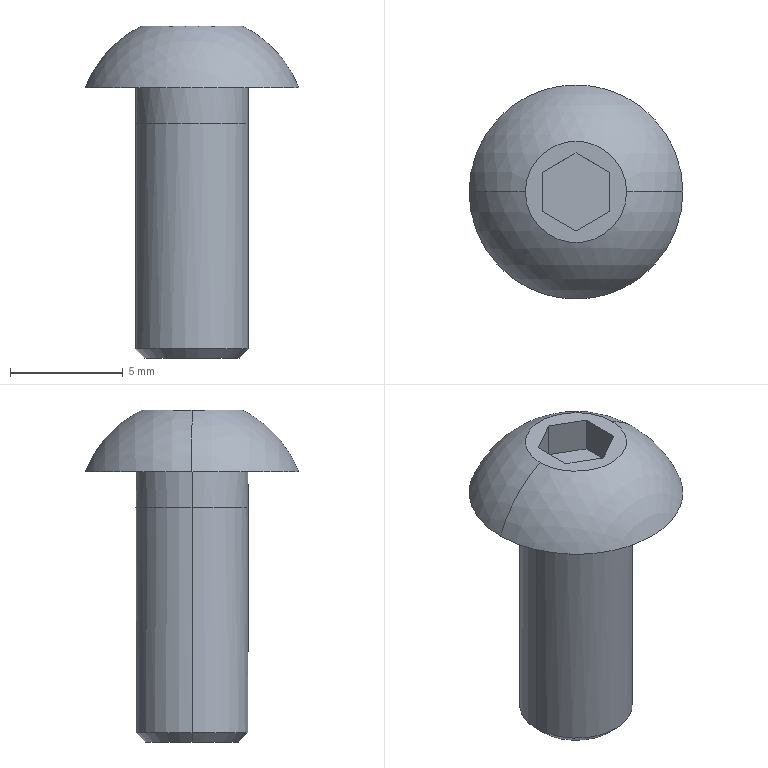Part | STEP file | button head socket screw ISO 7380 M5-12-A | 1 solid | 18 faces | box 9.5 x 9.5 x 14.75 mm | volume 352.491 mm3 | plane 10 | cylinder 4 | sphere 2 | cone 2 | commonest cylinder face diameters 5 x4
STEP:
#1=CARTESIAN_POINT('',(0.,0.,0.));
#2=DIRECTION('',(0.,0.,1.));
#3=DIRECTION('',(1.,0.,0.));
#4=AXIS2_PLACEMENT_3D('',#1,#2,#3);
#5=CARTESIAN_POINT('',(4.75,0.,0.));
#6=VERTEX_POINT('',#5);
#7=CARTESIAN_POINT('',(-4.75,0.,0.));
#8=VERTEX_POINT('',#7);
#9=CARTESIAN_POINT('',(0.,0.,0.));
#10=DIRECTION('',(0.,0.,1.));
#11=DIRECTION('',(1.,0.,0.));
#12=AXIS2_PLACEMENT_3D('',#9,#10,#11);
#13=CIRCLE('',#12,4.75);
#14=CARTESIAN_POINT('',(0.,0.,-1.807));
#15=DIRECTION('',(0.,1.,0.));
#16=DIRECTION('',(1.,0.,0.));
#17=AXIS2_PLACEMENT_3D('',#14,#15,#16);
#18=SPHERICAL_SURFACE('',#17,5.082);
#19=CARTESIAN_POINT('',(5.92,0.));
#20=CARTESIAN_POINT('',(5.92,0.04448));
#21=CARTESIAN_POINT('',(5.917,0.1335));
#22=CARTESIAN_POINT('',(5.907,0.2666));
#23=CARTESIAN_POINT('',(5.889,0.399));
#24=CARTESIAN_POINT('',(5.861,0.5301));
#25=CARTESIAN_POINT('',(5.82,0.6592));
#26=CARTESIAN_POINT('',(5.761,0.7852));
#27=CARTESIAN_POINT('',(5.677,0.9062));
#28=CARTESIAN_POINT('',(5.552,1.019));
#29=CARTESIAN_POINT('',(5.365,1.117));
#30=CARTESIAN_POINT('',(5.086,1.189));
#31=CARTESIAN_POINT('',(4.712,1.217));
#32=CARTESIAN_POINT('',(4.339,1.189));
#33=CARTESIAN_POINT('',(4.06,1.117));
#34=CARTESIAN_POINT('',(3.873,1.019));
#35=CARTESIAN_POINT('',(3.748,0.9062));
#36=CARTESIAN_POINT('',(3.663,0.7852));
#37=CARTESIAN_POINT('',(3.605,0.6592));
#38=CARTESIAN_POINT('',(3.564,0.5301));
#39=CARTESIAN_POINT('',(3.536,0.399));
#40=CARTESIAN_POINT('',(3.518,0.2666));
#41=CARTESIAN_POINT('',(3.507,0.1335));
#42=CARTESIAN_POINT('',(3.505,0.04448));
#43=CARTESIAN_POINT('',(3.505,0.));
#44=B_SPLINE_CURVE_WITH_KNOTS('',3,(#19,#20,#21,#22,#23,#24,#25,#26,#27,#28,#29,#30,#31,#32,#33,#34,#35,#36,#37,#38,#39,#40,#41,#42,#43),.UNSPECIFIED.,.F.,.F.,(4,1,1,1,1,1,1,1,1,1,1,1,1,1,1,1,1,1,1,1,1,1,4),(0.,0.1428,0.2856,0.4284,0.5712,0.714,0.8568,0.9996,1.142,1.285,1.428,1.571,1.714,1.856,1.999,2.142,2.285,2.428,2.57,2.713,2.856,2.999,3.142),.QUASI_UNIFORM_KNOTS.);
#45=(GEOMETRIC_REPRESENTATION_CONTEXT(2)PARAMETRIC_REPRESENTATION_CONTEXT()REPRESENTATION_CONTEXT('',''));
#46=DEFINITIONAL_REPRESENTATION('',(#44),#45);
#47=PCURVE('',#18,#46);
#48=CARTESIAN_POINT('',(2.5,0.,0.));
#49=DIRECTION('',(0.,0.,1.));
#50=DIRECTION('',(1.,0.,0.));
#51=AXIS2_PLACEMENT_3D('',#48,#49,#50);
#52=PLANE('',#51);
#53=CARTESIAN_POINT('',(-2.5,0.));
#54=DIRECTION('',(1.,0.));
#55=AXIS2_PLACEMENT_2D('',#53,#54);
#56=CIRCLE('',#55,4.75);
#57=(GEOMETRIC_REPRESENTATION_CONTEXT(2)PARAMETRIC_REPRESENTATION_CONTEXT()REPRESENTATION_CONTEXT('',''));
#58=DEFINITIONAL_REPRESENTATION('',(#56),#57);
#59=PCURVE('',#52,#58);
#60=SURFACE_CURVE('',#13,(#47,#59),.PCURVE_S1.);
#61=EDGE_CURVE('',#6,#8,#60,.T.);
#62=ORIENTED_EDGE('',*,*,#61,.T.);
#63=CARTESIAN_POINT('',(-2.25,0.,2.75));
#64=VERTEX_POINT('',#63);
#65=CARTESIAN_POINT('',(0.,0.,-1.807));
#66=DIRECTION('',(0.,1.,0.));
#67=DIRECTION('',(-1.,0.,0.));
#68=AXIS2_PLACEMENT_3D('',#65,#66,#67);
#69=CIRCLE('',#68,5.082);
#70=CARTESIAN_POINT('',(3.142,0.));
#71=DIRECTION('',(1.,0.));
#72=VECTOR('',#71,1.);
#73=LINE('',#70,#72);
#74=(GEOMETRIC_REPRESENTATION_CONTEXT(2)PARAMETRIC_REPRESENTATION_CONTEXT()REPRESENTATION_CONTEXT('',''));
#75=DEFINITIONAL_REPRESENTATION('',(#73),#74);
#76=PCURVE('',#18,#75);
#77=CARTESIAN_POINT('',(0.,0.,-1.807));
#78=DIRECTION('',(0.,1.,0.));
#79=DIRECTION('',(1.,0.,0.));
#80=AXIS2_PLACEMENT_3D('',#77,#78,#79);
#81=SPHERICAL_SURFACE('',#80,5.082);
#82=CARTESIAN_POINT('',(3.142,0.));
#83=DIRECTION('',(1.,0.));
#84=VECTOR('',#83,1.);
#85=LINE('',#82,#84);
#86=(GEOMETRIC_REPRESENTATION_CONTEXT(2)PARAMETRIC_REPRESENTATION_CONTEXT()REPRESENTATION_CONTEXT('',''));
#87=DEFINITIONAL_REPRESENTATION('',(#85),#86);
#88=PCURVE('',#81,#87);
#89=SURFACE_CURVE('',#69,(#76,#88),.PCURVE_S1.);
#90=EDGE_CURVE('',#8,#64,#89,.T.);
#91=ORIENTED_EDGE('',*,*,#90,.T.);
#92=CARTESIAN_POINT('',(2.25,0.,2.75));
#93=VERTEX_POINT('',#92);
#94=CARTESIAN_POINT('',(0.,0.,2.75));
#95=DIRECTION('',(0.,0.,1.));
#96=DIRECTION('',(1.,0.,0.));
#97=AXIS2_PLACEMENT_3D('',#94,#95,#96);
#98=CIRCLE('',#97,2.25);
#99=CARTESIAN_POINT('',(5.171,0.));
#100=CARTESIAN_POINT('',(5.171,0.02107));
#101=CARTESIAN_POINT('',(5.168,0.06322));
#102=CARTESIAN_POINT('',(5.156,0.1254));
#103=CARTESIAN_POINT('',(5.136,0.1855));
#104=CARTESIAN_POINT('',(5.107,0.2424));
#105=CARTESIAN_POINT('',(5.071,0.2951));
#106=CARTESIAN_POINT('',(5.026,0.3423));
#107=CARTESIAN_POINT('',(4.974,0.3829));
#108=CARTESIAN_POINT('',(4.916,0.4159));
#109=CARTESIAN_POINT('',(4.851,0.4403));
#110=CARTESIAN_POINT('',(4.783,0.4553));
#111=CARTESIAN_POINT('',(4.712,0.4603));
#112=CARTESIAN_POINT('',(4.642,0.4553));
#113=CARTESIAN_POINT('',(4.573,0.4403));
#114=CARTESIAN_POINT('',(4.509,0.4159));
#115=CARTESIAN_POINT('',(4.45,0.3829));
#116=CARTESIAN_POINT('',(4.398,0.3423));
#117=CARTESIAN_POINT('',(4.354,0.2951));
#118=CARTESIAN_POINT('',(4.317,0.2424));
#119=CARTESIAN_POINT('',(4.289,0.1855));
#120=CARTESIAN_POINT('',(4.269,0.1254));
#121=CARTESIAN_POINT('',(4.256,0.06322));
#122=CARTESIAN_POINT('',(4.254,0.02107));
#123=CARTESIAN_POINT('',(4.254,0.));
#124=B_SPLINE_CURVE_WITH_KNOTS('',3,(#99,#100,#101,#102,#103,#104,#105,#106,#107,#108,#109,#110,#111,#112,#113,#114,#115,#116,#117,#118,#119,#120,#121,#122,#123),.UNSPECIFIED.,.F.,.F.,(4,1,1,1,1,1,1,1,1,1,1,1,1,1,1,1,1,1,1,1,1,1,4),(0.,0.1428,0.2856,0.4284,0.5712,0.714,0.8568,0.9996,1.142,1.285,1.428,1.571,1.714,1.856,1.999,2.142,2.285,2.428,2.57,2.713,2.856,2.999,3.142),.QUASI_UNIFORM_KNOTS.);
#125=(GEOMETRIC_REPRESENTATION_CONTEXT(2)PARAMETRIC_REPRESENTATION_CONTEXT()REPRESENTATION_CONTEXT('',''));
#126=DEFINITIONAL_REPRESENTATION('',(#124),#125);
#127=PCURVE('',#18,#126);
#128=CARTESIAN_POINT('',(2.25,0.,2.75));
#129=DIRECTION('',(0.,0.,-1.));
#130=DIRECTION('',(-1.,0.,0.));
#131=AXIS2_PLACEMENT_3D('',#128,#129,#130);
#132=PLANE('',#131);
#133=CARTESIAN_POINT('',(0.,0.));
#134=CARTESIAN_POINT('',(0.,3.897));
#135=CARTESIAN_POINT('',(3.375,1.949));
#136=CARTESIAN_POINT('',(6.75,0.));
#137=CARTESIAN_POINT('',(3.375,-1.949));
#138=CARTESIAN_POINT('',(0.,-3.897));
#139=CARTESIAN_POINT('',(0.,0.));
#140=(BOUNDED_CURVE()B_SPLINE_CURVE(2,(#133,#134,#135,#136,#137,#138,#139),.UNSPECIFIED.,.T.,.F.)B_SPLINE_CURVE_WITH_KNOTS((1,2,2,2,2,1),(-2.094,0.,2.094,4.189,6.283,8.378),.UNSPECIFIED.)CURVE()GEOMETRIC_REPRESENTATION_ITEM()RATIONAL_B_SPLINE_CURVE((1.,0.5,1.,0.5,1.,0.5,1.))REPRESENTATION_ITEM(''));
#141=(GEOMETRIC_REPRESENTATION_CONTEXT(2)PARAMETRIC_REPRESENTATION_CONTEXT()REPRESENTATION_CONTEXT('',''));
#142=DEFINITIONAL_REPRESENTATION('',(#140),#141);
#143=PCURVE('',#132,#142);
#144=SURFACE_CURVE('',#98,(#127,#143),.PCURVE_S1.);
#145=EDGE_CURVE('',#93,#64,#144,.T.);
#146=ORIENTED_EDGE('',*,*,#145,.F.);
#147=CARTESIAN_POINT('',(0.,0.,-1.807));
#148=DIRECTION('',(0.,-1.,0.));
#149=DIRECTION('',(0.,0.,-1.));
#150=AXIS2_PLACEMENT_3D('',#147,#148,#149);
#151=CIRCLE('',#150,5.082);
#152=CARTESIAN_POINT('',(7.854,0.));
#153=DIRECTION('',(-1.,0.));
#154=VECTOR('',#153,1.);
#155=LINE('',#152,#154);
#156=(GEOMETRIC_REPRESENTATION_CONTEXT(2)PARAMETRIC_REPRESENTATION_CONTEXT()REPRESENTATION_CONTEXT('',''));
#157=DEFINITIONAL_REPRESENTATION('',(#155),#156);
#158=PCURVE('',#18,#157);
#159=CARTESIAN_POINT('',(7.854,0.));
#160=DIRECTION('',(-1.,0.));
#161=VECTOR('',#160,1.);
#162=LINE('',#159,#161);
#163=(GEOMETRIC_REPRESENTATION_CONTEXT(2)PARAMETRIC_REPRESENTATION_CONTEXT()REPRESENTATION_CONTEXT('',''));
#164=DEFINITIONAL_REPRESENTATION('',(#162),#163);
#165=PCURVE('',#81,#164);
#166=SURFACE_CURVE('',#151,(#158,#165),.PCURVE_S1.);
#167=EDGE_CURVE('',#6,#93,#166,.T.);
#168=ORIENTED_EDGE('',*,*,#167,.F.);
#169=EDGE_LOOP('',(#62,#91,#146,#168));
#170=FACE_BOUND('',#169,.T.);
#171=ADVANCED_FACE('',(#170),#18,.T.);
#172=CARTESIAN_POINT('',(-2.5,0.,-1.6));
#173=VERTEX_POINT('',#172);
#174=CARTESIAN_POINT('',(2.5,0.,-1.6));
#175=VERTEX_POINT('',#174);
#176=CARTESIAN_POINT('',(-2.5,0.,-1.6));
#177=CARTESIAN_POINT('',(-2.5,0.3272,-1.6));
#178=CARTESIAN_POINT('',(-2.435,0.6544,-1.6));
#179=CARTESIAN_POINT('',(-2.184,1.259,-1.6));
#180=CARTESIAN_POINT('',(-1.999,1.536,-1.6));
#181=CARTESIAN_POINT('',(-1.536,1.999,-1.6));
#182=CARTESIAN_POINT('',(-1.259,2.184,-1.6));
#183=CARTESIAN_POINT('',(-0.6544,2.435,-1.6));
#184=CARTESIAN_POINT('',(-0.3272,2.5,-1.6));
#185=CARTESIAN_POINT('',(0.3272,2.5,-1.6));
#186=CARTESIAN_POINT('',(0.6544,2.435,-1.6));
#187=CARTESIAN_POINT('',(1.259,2.184,-1.6));
#188=CARTESIAN_POINT('',(1.536,1.999,-1.6));
#189=CARTESIAN_POINT('',(1.999,1.536,-1.6));
#190=CARTESIAN_POINT('',(2.184,1.259,-1.6));
#191=CARTESIAN_POINT('',(2.435,0.6544,-1.6));
#192=CARTESIAN_POINT('',(2.5,0.3272,-1.6));
#193=CARTESIAN_POINT('',(2.5,0.,-1.6));
#194=B_SPLINE_CURVE_WITH_KNOTS('',3,(#176,#177,#178,#179,#180,#181,#182,#183,#184,#185,#186,#187,#188,#189,#190,#191,#192,#193),.UNSPECIFIED.,.F.,.F.,(4,2,2,2,2,2,2,2,4),(0.5,0.5625,0.625,0.6875,0.75,0.8125,0.875,0.9375,1.),.UNSPECIFIED.);
#195=CARTESIAN_POINT('',(0.,0.,2.75));
#196=DIRECTION('',(0.,0.,1.));
#197=DIRECTION('',(1.,0.,0.));
#198=AXIS2_PLACEMENT_3D('',#195,#196,#197);
#199=CYLINDRICAL_SURFACE('',#198,2.5);
#200=CARTESIAN_POINT('',(3.142,-4.35));
#201=CARTESIAN_POINT('',(0.,-4.35));
#202=B_SPLINE_CURVE_WITH_KNOTS('',1,(#200,#201),.UNSPECIFIED.,.F.,.F.,(2,2),(0.5,1.),.PIECEWISE_BEZIER_KNOTS.);
#203=(GEOMETRIC_REPRESENTATION_CONTEXT(2)PARAMETRIC_REPRESENTATION_CONTEXT()REPRESENTATION_CONTEXT('',''));
#204=DEFINITIONAL_REPRESENTATION('',(#202),#203);
#205=PCURVE('',#199,#204);
#206=CARTESIAN_POINT('',(0.,0.,2.75));
#207=DIRECTION('',(0.,0.,1.));
#208=DIRECTION('',(1.,0.,0.));
#209=AXIS2_PLACEMENT_3D('',#206,#207,#208);
#210=CYLINDRICAL_SURFACE('',#209,2.5);
#211=CARTESIAN_POINT('',(3.142,-4.35));
#212=CARTESIAN_POINT('',(0.,-4.35));
#213=B_SPLINE_CURVE_WITH_KNOTS('',1,(#211,#212),.UNSPECIFIED.,.F.,.F.,(2,2),(0.5,1.),.PIECEWISE_BEZIER_KNOTS.);
#214=(GEOMETRIC_REPRESENTATION_CONTEXT(2)PARAMETRIC_REPRESENTATION_CONTEXT()REPRESENTATION_CONTEXT('',''));
#215=DEFINITIONAL_REPRESENTATION('',(#213),#214);
#216=PCURVE('',#210,#215);
#217=SURFACE_CURVE('',#194,(#205,#216),.PCURVE_S1.);
#218=EDGE_CURVE('',#173,#175,#217,.T.);
#219=ORIENTED_EDGE('',*,*,#218,.F.);
#220=CARTESIAN_POINT('',(-2.5,0.,0.));
#221=VERTEX_POINT('',#220);
#222=CARTESIAN_POINT('',(-2.5,0.,2.75));
#223=DIRECTION('',(0.,0.,1.));
#224=VECTOR('',#223,1.);
#225=LINE('',#222,#224);
#226=CARTESIAN_POINT('',(3.142,0.));
#227=DIRECTION('',(0.,1.));
#228=VECTOR('',#227,1.);
#229=LINE('',#226,#228);
#230=(GEOMETRIC_REPRESENTATION_CONTEXT(2)PARAMETRIC_REPRESENTATION_CONTEXT()REPRESENTATION_CONTEXT('',''));
#231=DEFINITIONAL_REPRESENTATION('',(#229),#230);
#232=PCURVE('',#199,#231);
#233=CARTESIAN_POINT('',(0.,0.,2.75));
#234=DIRECTION('',(0.,0.,1.));
#235=DIRECTION('',(1.,0.,0.));
#236=AXIS2_PLACEMENT_3D('',#233,#234,#235);
#237=CYLINDRICAL_SURFACE('',#236,2.5);
#238=CARTESIAN_POINT('',(3.142,0.));
#239=DIRECTION('',(0.,1.));
#240=VECTOR('',#239,1.);
#241=LINE('',#238,#240);
#242=(GEOMETRIC_REPRESENTATION_CONTEXT(2)PARAMETRIC_REPRESENTATION_CONTEXT()REPRESENTATION_CONTEXT('',''));
#243=DEFINITIONAL_REPRESENTATION('',(#241),#242);
#244=PCURVE('',#237,#243);
#245=SURFACE_CURVE('',#225,(#232,#244),.PCURVE_S1.);
#246=EDGE_CURVE('',#173,#221,#245,.T.);
#247=ORIENTED_EDGE('',*,*,#246,.T.);
#248=CARTESIAN_POINT('',(2.5,0.,0.));
#249=VERTEX_POINT('',#248);
#250=CARTESIAN_POINT('',(0.,0.,0.));
#251=DIRECTION('',(0.,0.,1.));
#252=DIRECTION('',(1.,0.,0.));
#253=AXIS2_PLACEMENT_3D('',#250,#251,#252);
#254=CIRCLE('',#253,2.5);
#255=CARTESIAN_POINT('',(0.,-2.75));
#256=DIRECTION('',(1.,0.));
#257=VECTOR('',#256,1.);
#258=LINE('',#255,#257);
#259=(GEOMETRIC_REPRESENTATION_CONTEXT(2)PARAMETRIC_REPRESENTATION_CONTEXT()REPRESENTATION_CONTEXT('',''));
#260=DEFINITIONAL_REPRESENTATION('',(#258),#259);
#261=PCURVE('',#199,#260);
#262=CARTESIAN_POINT('',(-2.5,0.));
#263=DIRECTION('',(1.,0.));
#264=AXIS2_PLACEMENT_2D('',#262,#263);
#265=CIRCLE('',#264,2.5);
#266=(GEOMETRIC_REPRESENTATION_CONTEXT(2)PARAMETRIC_REPRESENTATION_CONTEXT()REPRESENTATION_CONTEXT('',''));
#267=DEFINITIONAL_REPRESENTATION('',(#265),#266);
#268=PCURVE('',#52,#267);
#269=SURFACE_CURVE('',#254,(#261,#268),.PCURVE_S1.);
#270=EDGE_CURVE('',#249,#221,#269,.T.);
#271=ORIENTED_EDGE('',*,*,#270,.F.);
#272=CARTESIAN_POINT('',(2.5,0.,2.75));
#273=DIRECTION('',(0.,0.,1.));
#274=VECTOR('',#273,1.);
#275=LINE('',#272,#274);
#276=CARTESIAN_POINT('',(0.,0.));
#277=DIRECTION('',(0.,1.));
#278=VECTOR('',#277,1.);
#279=LINE('',#276,#278);
#280=(GEOMETRIC_REPRESENTATION_CONTEXT(2)PARAMETRIC_REPRESENTATION_CONTEXT()REPRESENTATION_CONTEXT('',''));
#281=DEFINITIONAL_REPRESENTATION('',(#279),#280);
#282=PCURVE('',#199,#281);
#283=CARTESIAN_POINT('',(6.283,0.));
#284=DIRECTION('',(0.,1.));
#285=VECTOR('',#284,1.);
#286=LINE('',#283,#285);
#287=(GEOMETRIC_REPRESENTATION_CONTEXT(2)PARAMETRIC_REPRESENTATION_CONTEXT()REPRESENTATION_CONTEXT('',''));
#288=DEFINITIONAL_REPRESENTATION('',(#286),#287);
#289=PCURVE('',#237,#288);
#290=SURFACE_CURVE('',#275,(#282,#289),.PCURVE_S1.);
#291=EDGE_CURVE('',#175,#249,#290,.T.);
#292=ORIENTED_EDGE('',*,*,#291,.F.);
#293=EDGE_LOOP('',(#219,#247,#271,#292));
#294=FACE_BOUND('',#293,.T.);
#295=ADVANCED_FACE('',(#294),#199,.T.);
#296=CARTESIAN_POINT('',(2.1,0.,-12.));
#297=VERTEX_POINT('',#296);
#298=CARTESIAN_POINT('',(-2.1,0.,-12.));
#299=VERTEX_POINT('',#298);
#300=CARTESIAN_POINT('',(0.,0.,-12.));
#301=DIRECTION('',(0.,0.,1.));
#302=DIRECTION('',(1.,0.,0.));
#303=AXIS2_PLACEMENT_3D('',#300,#301,#302);
#304=CIRCLE('',#303,2.1);
#305=CARTESIAN_POINT('',(0.,0.,-12.));
#306=DIRECTION('',(0.,0.,1.));
#307=DIRECTION('',(1.,0.,0.));
#308=AXIS2_PLACEMENT_3D('',#305,#306,#307);
#309=CONICAL_SURFACE('',#308,2.1,0.7854);
#310=CARTESIAN_POINT('',(0.,0.));
#311=DIRECTION('',(1.,0.));
#312=VECTOR('',#311,1.);
#313=LINE('',#310,#312);
#314=(GEOMETRIC_REPRESENTATION_CONTEXT(2)PARAMETRIC_REPRESENTATION_CONTEXT()REPRESENTATION_CONTEXT('',''));
#315=DEFINITIONAL_REPRESENTATION('',(#313),#314);
#316=PCURVE('',#309,#315);
#317=CARTESIAN_POINT('',(0.,0.,-12.));
#318=DIRECTION('',(0.,0.,1.));
#319=DIRECTION('',(1.,0.,0.));
#320=AXIS2_PLACEMENT_3D('',#317,#318,#319);
#321=PLANE('',#320);
#322=CARTESIAN_POINT('',(0.,0.));
#323=DIRECTION('',(1.,0.));
#324=AXIS2_PLACEMENT_2D('',#322,#323);
#325=CIRCLE('',#324,2.1);
#326=(GEOMETRIC_REPRESENTATION_CONTEXT(2)PARAMETRIC_REPRESENTATION_CONTEXT()REPRESENTATION_CONTEXT('',''));
#327=DEFINITIONAL_REPRESENTATION('',(#325),#326);
#328=PCURVE('',#321,#327);
#329=SURFACE_CURVE('',#304,(#316,#328),.PCURVE_S1.);
#330=EDGE_CURVE('',#297,#299,#329,.T.);
#331=ORIENTED_EDGE('',*,*,#330,.T.);
#332=CARTESIAN_POINT('',(-2.5,0.,-11.6));
#333=VERTEX_POINT('',#332);
#334=CARTESIAN_POINT('',(-2.1,0.,-12.));
#335=DIRECTION('',(-0.7071,0.,0.7071));
#336=VECTOR('',#335,1.);
#337=LINE('',#334,#336);
#338=CARTESIAN_POINT('',(3.142,0.));
#339=DIRECTION('',(0.,1.));
#340=VECTOR('',#339,1.);
#341=LINE('',#338,#340);
#342=(GEOMETRIC_REPRESENTATION_CONTEXT(2)PARAMETRIC_REPRESENTATION_CONTEXT()REPRESENTATION_CONTEXT('',''));
#343=DEFINITIONAL_REPRESENTATION('',(#341),#342);
#344=PCURVE('',#309,#343);
#345=CARTESIAN_POINT('',(0.,0.,-12.));
#346=DIRECTION('',(0.,0.,1.));
#347=DIRECTION('',(1.,0.,0.));
#348=AXIS2_PLACEMENT_3D('',#345,#346,#347);
#349=CONICAL_SURFACE('',#348,2.1,0.7854);
#350=CARTESIAN_POINT('',(3.142,0.));
#351=DIRECTION('',(0.,1.));
#352=VECTOR('',#351,1.);
#353=LINE('',#350,#352);
#354=(GEOMETRIC_REPRESENTATION_CONTEXT(2)PARAMETRIC_REPRESENTATION_CONTEXT()REPRESENTATION_CONTEXT('',''));
#355=DEFINITIONAL_REPRESENTATION('',(#353),#354);
#356=PCURVE('',#349,#355);
#357=SURFACE_CURVE('',#337,(#344,#356),.PCURVE_S1.);
#358=EDGE_CURVE('',#299,#333,#357,.T.);
#359=ORIENTED_EDGE('',*,*,#358,.T.);
#360=CARTESIAN_POINT('',(2.5,0.,-11.6));
#361=VERTEX_POINT('',#360);
#362=CARTESIAN_POINT('',(0.,0.,-11.6));
#363=DIRECTION('',(0.,0.,1.));
#364=DIRECTION('',(1.,0.,0.));
#365=AXIS2_PLACEMENT_3D('',#362,#363,#364);
#366=CIRCLE('',#365,2.5);
#367=CARTESIAN_POINT('',(0.,0.4));
#368=DIRECTION('',(1.,0.));
#369=VECTOR('',#368,1.);
#370=LINE('',#367,#369);
#371=(GEOMETRIC_REPRESENTATION_CONTEXT(2)PARAMETRIC_REPRESENTATION_CONTEXT()REPRESENTATION_CONTEXT('',''));
#372=DEFINITIONAL_REPRESENTATION('',(#370),#371);
#373=PCURVE('',#309,#372);
#374=CARTESIAN_POINT('',(0.,-14.35));
#375=DIRECTION('',(1.,0.));
#376=VECTOR('',#375,1.);
#377=LINE('',#374,#376);
#378=(GEOMETRIC_REPRESENTATION_CONTEXT(2)PARAMETRIC_REPRESENTATION_CONTEXT()REPRESENTATION_CONTEXT('',''));
#379=DEFINITIONAL_REPRESENTATION('',(#377),#378);
#380=PCURVE('',#210,#379);
#381=SURFACE_CURVE('',#366,(#373,#380),.PCURVE_S1.);
#382=EDGE_CURVE('',#361,#333,#381,.T.);
#383=ORIENTED_EDGE('',*,*,#382,.F.);
#384=CARTESIAN_POINT('',(2.1,0.,-12.));
#385=DIRECTION('',(0.7071,0.,0.7071));
#386=VECTOR('',#385,1.);
#387=LINE('',#384,#386);
#388=CARTESIAN_POINT('',(0.,0.));
#389=DIRECTION('',(0.,1.));
#390=VECTOR('',#389,1.);
#391=LINE('',#388,#390);
#392=(GEOMETRIC_REPRESENTATION_CONTEXT(2)PARAMETRIC_REPRESENTATION_CONTEXT()REPRESENTATION_CONTEXT('',''));
#393=DEFINITIONAL_REPRESENTATION('',(#391),#392);
#394=PCURVE('',#309,#393);
#395=CARTESIAN_POINT('',(6.283,0.));
#396=DIRECTION('',(0.,1.));
#397=VECTOR('',#396,1.);
#398=LINE('',#395,#397);
#399=(GEOMETRIC_REPRESENTATION_CONTEXT(2)PARAMETRIC_REPRESENTATION_CONTEXT()REPRESENTATION_CONTEXT('',''));
#400=DEFINITIONAL_REPRESENTATION('',(#398),#399);
#401=PCURVE('',#349,#400);
#402=SURFACE_CURVE('',#387,(#394,#401),.PCURVE_S1.);
#403=EDGE_CURVE('',#297,#361,#402,.T.);
#404=ORIENTED_EDGE('',*,*,#403,.F.);
#405=EDGE_LOOP('',(#331,#359,#383,#404));
#406=FACE_BOUND('',#405,.T.);
#407=ADVANCED_FACE('',(#406),#309,.T.);
#408=ORIENTED_EDGE('',*,*,#382,.T.);
#409=CARTESIAN_POINT('',(-2.5,0.,2.75));
#410=DIRECTION('',(0.,0.,1.));
#411=VECTOR('',#410,1.);
#412=LINE('',#409,#411);
#413=CARTESIAN_POINT('',(3.142,0.));
#414=DIRECTION('',(0.,1.));
#415=VECTOR('',#414,1.);
#416=LINE('',#413,#415);
#417=(GEOMETRIC_REPRESENTATION_CONTEXT(2)PARAMETRIC_REPRESENTATION_CONTEXT()REPRESENTATION_CONTEXT('',''));
#418=DEFINITIONAL_REPRESENTATION('',(#416),#417);
#419=PCURVE('',#210,#418);
#420=CARTESIAN_POINT('',(0.,0.,2.75));
#421=DIRECTION('',(0.,0.,1.));
#422=DIRECTION('',(1.,0.,0.));
#423=AXIS2_PLACEMENT_3D('',#420,#421,#422);
#424=CYLINDRICAL_SURFACE('',#423,2.5);
#425=CARTESIAN_POINT('',(3.142,0.));
#426=DIRECTION('',(0.,1.));
#427=VECTOR('',#426,1.);
#428=LINE('',#425,#427);
#429=(GEOMETRIC_REPRESENTATION_CONTEXT(2)PARAMETRIC_REPRESENTATION_CONTEXT()REPRESENTATION_CONTEXT('',''));
#430=DEFINITIONAL_REPRESENTATION('',(#428),#429);
#431=PCURVE('',#424,#430);
#432=SURFACE_CURVE('',#412,(#419,#431),.PCURVE_S1.);
#433=EDGE_CURVE('',#333,#173,#432,.T.);
#434=ORIENTED_EDGE('',*,*,#433,.T.);
#435=ORIENTED_EDGE('',*,*,#218,.T.);
#436=CARTESIAN_POINT('',(2.5,0.,2.75));
#437=DIRECTION('',(0.,0.,1.));
#438=VECTOR('',#437,1.);
#439=LINE('',#436,#438);
#440=CARTESIAN_POINT('',(0.,0.));
#441=DIRECTION('',(0.,1.));
#442=VECTOR('',#441,1.);
#443=LINE('',#440,#442);
#444=(GEOMETRIC_REPRESENTATION_CONTEXT(2)PARAMETRIC_REPRESENTATION_CONTEXT()REPRESENTATION_CONTEXT('',''));
#445=DEFINITIONAL_REPRESENTATION('',(#443),#444);
#446=PCURVE('',#210,#445);
#447=CARTESIAN_POINT('',(6.283,0.));
#448=DIRECTION('',(0.,1.));
#449=VECTOR('',#448,1.);
#450=LINE('',#447,#449);
#451=(GEOMETRIC_REPRESENTATION_CONTEXT(2)PARAMETRIC_REPRESENTATION_CONTEXT()REPRESENTATION_CONTEXT('',''));
#452=DEFINITIONAL_REPRESENTATION('',(#450),#451);
#453=PCURVE('',#424,#452);
#454=SURFACE_CURVE('',#439,(#446,#453),.PCURVE_S1.);
#455=EDGE_CURVE('',#361,#175,#454,.T.);
#456=ORIENTED_EDGE('',*,*,#455,.F.);
#457=EDGE_LOOP('',(#408,#434,#435,#456));
#458=FACE_BOUND('',#457,.T.);
#459=ADVANCED_FACE('',(#458),#210,.T.);
#460=ORIENTED_EDGE('',*,*,#433,.F.);
#461=CARTESIAN_POINT('',(0.,0.,-11.6));
#462=DIRECTION('',(0.,0.,1.));
#463=DIRECTION('',(1.,0.,0.));
#464=AXIS2_PLACEMENT_3D('',#461,#462,#463);
#465=CIRCLE('',#464,2.5);
#466=CARTESIAN_POINT('',(0.,-14.35));
#467=DIRECTION('',(1.,0.));
#468=VECTOR('',#467,1.);
#469=LINE('',#466,#468);
#470=(GEOMETRIC_REPRESENTATION_CONTEXT(2)PARAMETRIC_REPRESENTATION_CONTEXT()REPRESENTATION_CONTEXT('',''));
#471=DEFINITIONAL_REPRESENTATION('',(#469),#470);
#472=PCURVE('',#424,#471);
#473=CARTESIAN_POINT('',(0.,0.4));
#474=DIRECTION('',(1.,0.));
#475=VECTOR('',#474,1.);
#476=LINE('',#473,#475);
#477=(GEOMETRIC_REPRESENTATION_CONTEXT(2)PARAMETRIC_REPRESENTATION_CONTEXT()REPRESENTATION_CONTEXT('',''));
#478=DEFINITIONAL_REPRESENTATION('',(#476),#477);
#479=PCURVE('',#349,#478);
#480=SURFACE_CURVE('',#465,(#472,#479),.PCURVE_S1.);
#481=EDGE_CURVE('',#333,#361,#480,.T.);
#482=ORIENTED_EDGE('',*,*,#481,.T.);
#483=ORIENTED_EDGE('',*,*,#455,.T.);
#484=CARTESIAN_POINT('',(2.5,0.,-1.6));
#485=CARTESIAN_POINT('',(2.5,-0.3272,-1.6));
#486=CARTESIAN_POINT('',(2.435,-0.6544,-1.6));
#487=CARTESIAN_POINT('',(2.184,-1.259,-1.6));
#488=CARTESIAN_POINT('',(1.999,-1.536,-1.6));
#489=CARTESIAN_POINT('',(1.536,-1.999,-1.6));
#490=CARTESIAN_POINT('',(1.259,-2.184,-1.6));
#491=CARTESIAN_POINT('',(0.6544,-2.435,-1.6));
#492=CARTESIAN_POINT('',(0.3272,-2.5,-1.6));
#493=CARTESIAN_POINT('',(-0.3272,-2.5,-1.6));
#494=CARTESIAN_POINT('',(-0.6544,-2.435,-1.6));
#495=CARTESIAN_POINT('',(-1.259,-2.184,-1.6));
#496=CARTESIAN_POINT('',(-1.536,-1.999,-1.6));
#497=CARTESIAN_POINT('',(-1.999,-1.536,-1.6));
#498=CARTESIAN_POINT('',(-2.184,-1.259,-1.6));
#499=CARTESIAN_POINT('',(-2.435,-0.6544,-1.6));
#500=CARTESIAN_POINT('',(-2.5,-0.3272,-1.6));
#501=CARTESIAN_POINT('',(-2.5,0.,-1.6));
#502=B_SPLINE_CURVE_WITH_KNOTS('',3,(#484,#485,#486,#487,#488,#489,#490,#491,#492,#493,#494,#495,#496,#497,#498,#499,#500,#501),.UNSPECIFIED.,.F.,.F.,(4,2,2,2,2,2,2,2,4),(0.,0.0625,0.125,0.1875,0.25,0.3125,0.375,0.4375,0.5),.UNSPECIFIED.);
#503=CARTESIAN_POINT('',(6.283,-4.35));
#504=CARTESIAN_POINT('',(3.142,-4.35));
#505=B_SPLINE_CURVE_WITH_KNOTS('',1,(#503,#504),.UNSPECIFIED.,.F.,.F.,(2,2),(0.,0.5),.PIECEWISE_BEZIER_KNOTS.);
#506=(GEOMETRIC_REPRESENTATION_CONTEXT(2)PARAMETRIC_REPRESENTATION_CONTEXT()REPRESENTATION_CONTEXT('',''));
#507=DEFINITIONAL_REPRESENTATION('',(#505),#506);
#508=PCURVE('',#424,#507);
#509=CARTESIAN_POINT('',(6.283,-4.35));
#510=CARTESIAN_POINT('',(3.142,-4.35));
#511=B_SPLINE_CURVE_WITH_KNOTS('',1,(#509,#510),.UNSPECIFIED.,.F.,.F.,(2,2),(0.,0.5),.PIECEWISE_BEZIER_KNOTS.);
#512=(GEOMETRIC_REPRESENTATION_CONTEXT(2)PARAMETRIC_REPRESENTATION_CONTEXT()REPRESENTATION_CONTEXT('',''));
#513=DEFINITIONAL_REPRESENTATION('',(#511),#512);
#514=PCURVE('',#237,#513);
#515=SURFACE_CURVE('',#502,(#508,#514),.PCURVE_S1.);
#516=EDGE_CURVE('',#175,#173,#515,.T.);
#517=ORIENTED_EDGE('',*,*,#516,.T.);
#518=EDGE_LOOP('',(#460,#482,#483,#517));
#519=FACE_BOUND('',#518,.T.);
#520=ADVANCED_FACE('',(#519),#424,.T.);
#521=ORIENTED_EDGE('',*,*,#145,.T.);
#522=CARTESIAN_POINT('',(0.,0.,2.75));
#523=DIRECTION('',(0.,0.,1.));
#524=DIRECTION('',(1.,0.,0.));
#525=AXIS2_PLACEMENT_3D('',#522,#523,#524);
#526=CIRCLE('',#525,2.25);
#527=CARTESIAN_POINT('',(0.,0.));
#528=CARTESIAN_POINT('',(0.,3.897));
#529=CARTESIAN_POINT('',(3.375,1.949));
#530=CARTESIAN_POINT('',(6.75,0.));
#531=CARTESIAN_POINT('',(3.375,-1.949));
#532=CARTESIAN_POINT('',(0.,-3.897));
#533=CARTESIAN_POINT('',(0.,0.));
#534=(BOUNDED_CURVE()B_SPLINE_CURVE(2,(#527,#528,#529,#530,#531,#532,#533),.UNSPECIFIED.,.T.,.F.)B_SPLINE_CURVE_WITH_KNOTS((1,2,2,2,2,1),(-2.094,0.,2.094,4.189,6.283,8.378),.UNSPECIFIED.)CURVE()GEOMETRIC_REPRESENTATION_ITEM()RATIONAL_B_SPLINE_CURVE((1.,0.5,1.,0.5,1.,0.5,1.))REPRESENTATION_ITEM(''));
#535=(GEOMETRIC_REPRESENTATION_CONTEXT(2)PARAMETRIC_REPRESENTATION_CONTEXT()REPRESENTATION_CONTEXT('',''));
#536=DEFINITIONAL_REPRESENTATION('',(#534),#535);
#537=PCURVE('',#132,#536);
#538=CARTESIAN_POINT('',(4.254,0.));
#539=CARTESIAN_POINT('',(4.254,-0.02107));
#540=CARTESIAN_POINT('',(4.256,-0.06322));
#541=CARTESIAN_POINT('',(4.269,-0.1254));
#542=CARTESIAN_POINT('',(4.289,-0.1855));
#543=CARTESIAN_POINT('',(4.317,-0.2424));
#544=CARTESIAN_POINT('',(4.354,-0.2951));
#545=CARTESIAN_POINT('',(4.398,-0.3423));
#546=CARTESIAN_POINT('',(4.45,-0.3829));
#547=CARTESIAN_POINT('',(4.509,-0.4159));
#548=CARTESIAN_POINT('',(4.573,-0.4403));
#549=CARTESIAN_POINT('',(4.642,-0.4553));
#550=CARTESIAN_POINT('',(4.712,-0.4603));
#551=CARTESIAN_POINT('',(4.783,-0.4553));
#552=CARTESIAN_POINT('',(4.851,-0.4403));
#553=CARTESIAN_POINT('',(4.916,-0.4159));
#554=CARTESIAN_POINT('',(4.974,-0.3829));
#555=CARTESIAN_POINT('',(5.026,-0.3423));
#556=CARTESIAN_POINT('',(5.071,-0.2951));
#557=CARTESIAN_POINT('',(5.107,-0.2424));
#558=CARTESIAN_POINT('',(5.136,-0.1855));
#559=CARTESIAN_POINT('',(5.156,-0.1254));
#560=CARTESIAN_POINT('',(5.168,-0.06322));
#561=CARTESIAN_POINT('',(5.171,-0.02107));
#562=CARTESIAN_POINT('',(5.171,0.));
#563=B_SPLINE_CURVE_WITH_KNOTS('',3,(#538,#539,#540,#541,#542,#543,#544,#545,#546,#547,#548,#549,#550,#551,#552,#553,#554,#555,#556,#557,#558,#559,#560,#561,#562),.UNSPECIFIED.,.F.,.F.,(4,1,1,1,1,1,1,1,1,1,1,1,1,1,1,1,1,1,1,1,1,1,4),(3.142,3.284,3.427,3.57,3.713,3.856,3.998,4.141,4.284,4.427,4.57,4.712,4.855,4.998,5.141,5.284,5.426,5.569,5.712,5.855,5.998,6.14,6.283),.QUASI_UNIFORM_KNOTS.);
#564=(GEOMETRIC_REPRESENTATION_CONTEXT(2)PARAMETRIC_REPRESENTATION_CONTEXT()REPRESENTATION_CONTEXT('',''));
#565=DEFINITIONAL_REPRESENTATION('',(#563),#564);
#566=PCURVE('',#81,#565);
#567=SURFACE_CURVE('',#526,(#537,#566),.PCURVE_S1.);
#568=EDGE_CURVE('',#64,#93,#567,.T.);
#569=ORIENTED_EDGE('',*,*,#568,.T.);
#570=EDGE_LOOP('',(#521,#569));
#571=FACE_BOUND('',#570,.T.);
#572=CARTESIAN_POINT('',(1.5,-0.866,2.75));
#573=VERTEX_POINT('',#572);
#574=CARTESIAN_POINT('',(1.5,0.866,2.75));
#575=VERTEX_POINT('',#574);
#576=CARTESIAN_POINT('',(1.5,0.,2.75));
#577=DIRECTION('',(0.,1.,0.));
#578=VECTOR('',#577,1.);
#579=LINE('',#576,#578);
#580=CARTESIAN_POINT('',(0.75,0.));
#581=DIRECTION('',(0.,1.));
#582=VECTOR('',#581,1.);
#583=LINE('',#580,#582);
#584=(GEOMETRIC_REPRESENTATION_CONTEXT(2)PARAMETRIC_REPRESENTATION_CONTEXT()REPRESENTATION_CONTEXT('',''));
#585=DEFINITIONAL_REPRESENTATION('',(#583),#584);
#586=PCURVE('',#132,#585);
#587=CARTESIAN_POINT('',(1.5,-0.866,21.142));
#588=DIRECTION('',(-1.,0.,0.));
#589=DIRECTION('',(0.,-1.,0.));
#590=AXIS2_PLACEMENT_3D('',#587,#588,#589);
#591=PLANE('',#590);
#592=CARTESIAN_POINT('',(-0.866,-18.392));
#593=DIRECTION('',(-1.,0.));
#594=VECTOR('',#593,1.);
#595=LINE('',#592,#594);
#596=(GEOMETRIC_REPRESENTATION_CONTEXT(2)PARAMETRIC_REPRESENTATION_CONTEXT()REPRESENTATION_CONTEXT('',''));
#597=DEFINITIONAL_REPRESENTATION('',(#595),#596);
#598=PCURVE('',#591,#597);
#599=SURFACE_CURVE('',#579,(#586,#598),.PCURVE_S1.);
#600=EDGE_CURVE('',#573,#575,#599,.T.);
#601=ORIENTED_EDGE('',*,*,#600,.F.);
#602=CARTESIAN_POINT('',(0.,-1.732,2.75));
#603=VERTEX_POINT('',#602);
#604=CARTESIAN_POINT('',(2.438,-0.3248,2.75));
#605=DIRECTION('',(0.866,0.5,0.));
#606=VECTOR('',#605,1.);
#607=LINE('',#604,#606);
#608=CARTESIAN_POINT('',(-0.1875,-0.3248));
#609=DIRECTION('',(-0.866,0.5));
#610=VECTOR('',#609,1.);
#611=LINE('',#608,#610);
#612=(GEOMETRIC_REPRESENTATION_CONTEXT(2)PARAMETRIC_REPRESENTATION_CONTEXT()REPRESENTATION_CONTEXT('',''));
#613=DEFINITIONAL_REPRESENTATION('',(#611),#612);
#614=PCURVE('',#132,#613);
#615=CARTESIAN_POINT('',(0.,-1.732,21.142));
#616=DIRECTION('',(-0.5,0.866,0.));
#617=DIRECTION('',(-0.866,-0.5,0.));
#618=AXIS2_PLACEMENT_3D('',#615,#616,#617);
#619=PLANE('',#618);
#620=CARTESIAN_POINT('',(-2.815,-18.392));
#621=DIRECTION('',(-1.,0.));
#622=VECTOR('',#621,1.);
#623=LINE('',#620,#622);
#624=(GEOMETRIC_REPRESENTATION_CONTEXT(2)PARAMETRIC_REPRESENTATION_CONTEXT()REPRESENTATION_CONTEXT('',''));
#625=DEFINITIONAL_REPRESENTATION('',(#623),#624);
#626=PCURVE('',#619,#625);
#627=SURFACE_CURVE('',#607,(#614,#626),.PCURVE_S1.);
#628=EDGE_CURVE('',#603,#573,#627,.T.);
#629=ORIENTED_EDGE('',*,*,#628,.F.);
#630=CARTESIAN_POINT('',(-1.5,-0.866,2.75));
#631=VERTEX_POINT('',#630);
#632=CARTESIAN_POINT('',(0.9375,-2.273,2.75));
#633=DIRECTION('',(0.866,-0.5,0.));
#634=VECTOR('',#633,1.);
#635=LINE('',#632,#634);
#636=CARTESIAN_POINT('',(1.312,-2.273));
#637=DIRECTION('',(-0.866,-0.5));
#638=VECTOR('',#637,1.);
#639=LINE('',#636,#638);
#640=(GEOMETRIC_REPRESENTATION_CONTEXT(2)PARAMETRIC_REPRESENTATION_CONTEXT()REPRESENTATION_CONTEXT('',''));
#641=DEFINITIONAL_REPRESENTATION('',(#639),#640);
#642=PCURVE('',#132,#641);
#643=CARTESIAN_POINT('',(-1.5,-0.866,21.142));
#644=DIRECTION('',(0.5,0.866,0.));
#645=DIRECTION('',(-0.866,0.5,0.));
#646=AXIS2_PLACEMENT_3D('',#643,#644,#645);
#647=PLANE('',#646);
#648=CARTESIAN_POINT('',(-2.815,-18.392));
#649=DIRECTION('',(-1.,0.));
#650=VECTOR('',#649,1.);
#651=LINE('',#648,#650);
#652=(GEOMETRIC_REPRESENTATION_CONTEXT(2)PARAMETRIC_REPRESENTATION_CONTEXT()REPRESENTATION_CONTEXT('',''));
#653=DEFINITIONAL_REPRESENTATION('',(#651),#652);
#654=PCURVE('',#647,#653);
#655=SURFACE_CURVE('',#635,(#642,#654),.PCURVE_S1.);
#656=EDGE_CURVE('',#631,#603,#655,.T.);
#657=ORIENTED_EDGE('',*,*,#656,.F.);
#658=CARTESIAN_POINT('',(-1.5,0.866,2.75));
#659=VERTEX_POINT('',#658);
#660=CARTESIAN_POINT('',(-1.5,0.,2.75));
#661=DIRECTION('',(0.,-1.,0.));
#662=VECTOR('',#661,1.);
#663=LINE('',#660,#662);
#664=CARTESIAN_POINT('',(3.75,0.));
#665=DIRECTION('',(0.,-1.));
#666=VECTOR('',#665,1.);
#667=LINE('',#664,#666);
#668=(GEOMETRIC_REPRESENTATION_CONTEXT(2)PARAMETRIC_REPRESENTATION_CONTEXT()REPRESENTATION_CONTEXT('',''));
#669=DEFINITIONAL_REPRESENTATION('',(#667),#668);
#670=PCURVE('',#132,#669);
#671=CARTESIAN_POINT('',(-1.5,0.866,21.142));
#672=DIRECTION('',(1.,0.,0.));
#673=DIRECTION('',(0.,1.,0.));
#674=AXIS2_PLACEMENT_3D('',#671,#672,#673);
#675=PLANE('',#674);
#676=CARTESIAN_POINT('',(-0.866,-18.392));
#677=DIRECTION('',(-1.,0.));
#678=VECTOR('',#677,1.);
#679=LINE('',#676,#678);
#680=(GEOMETRIC_REPRESENTATION_CONTEXT(2)PARAMETRIC_REPRESENTATION_CONTEXT()REPRESENTATION_CONTEXT('',''));
#681=DEFINITIONAL_REPRESENTATION('',(#679),#680);
#682=PCURVE('',#675,#681);
#683=SURFACE_CURVE('',#663,(#670,#682),.PCURVE_S1.);
#684=EDGE_CURVE('',#659,#631,#683,.T.);
#685=ORIENTED_EDGE('',*,*,#684,.F.);
#686=CARTESIAN_POINT('',(0.,1.732,2.75));
#687=VERTEX_POINT('',#686);
#688=CARTESIAN_POINT('',(0.9375,2.273,2.75));
#689=DIRECTION('',(-0.866,-0.5,0.));
#690=VECTOR('',#689,1.);
#691=LINE('',#688,#690);
#692=CARTESIAN_POINT('',(1.312,2.273));
#693=DIRECTION('',(0.866,-0.5));
#694=VECTOR('',#693,1.);
#695=LINE('',#692,#694);
#696=(GEOMETRIC_REPRESENTATION_CONTEXT(2)PARAMETRIC_REPRESENTATION_CONTEXT()REPRESENTATION_CONTEXT('',''));
#697=DEFINITIONAL_REPRESENTATION('',(#695),#696);
#698=PCURVE('',#132,#697);
#699=CARTESIAN_POINT('',(0.,1.732,21.142));
#700=DIRECTION('',(0.5,-0.866,0.));
#701=DIRECTION('',(0.866,0.5,0.));
#702=AXIS2_PLACEMENT_3D('',#699,#700,#701);
#703=PLANE('',#702);
#704=CARTESIAN_POINT('',(1.083,-18.392));
#705=DIRECTION('',(-1.,0.));
#706=VECTOR('',#705,1.);
#707=LINE('',#704,#706);
#708=(GEOMETRIC_REPRESENTATION_CONTEXT(2)PARAMETRIC_REPRESENTATION_CONTEXT()REPRESENTATION_CONTEXT('',''));
#709=DEFINITIONAL_REPRESENTATION('',(#707),#708);
#710=PCURVE('',#703,#709);
#711=SURFACE_CURVE('',#691,(#698,#710),.PCURVE_S1.);
#712=EDGE_CURVE('',#687,#659,#711,.T.);
#713=ORIENTED_EDGE('',*,*,#712,.F.);
#714=CARTESIAN_POINT('',(2.438,0.3248,2.75));
#715=DIRECTION('',(-0.866,0.5,0.));
#716=VECTOR('',#715,1.);
#717=LINE('',#714,#716);
#718=CARTESIAN_POINT('',(-0.1875,0.3248));
#719=DIRECTION('',(0.866,0.5));
#720=VECTOR('',#719,1.);
#721=LINE('',#718,#720);
#722=(GEOMETRIC_REPRESENTATION_CONTEXT(2)PARAMETRIC_REPRESENTATION_CONTEXT()REPRESENTATION_CONTEXT('',''));
#723=DEFINITIONAL_REPRESENTATION('',(#721),#722);
#724=PCURVE('',#132,#723);
#725=CARTESIAN_POINT('',(1.5,0.866,21.142));
#726=DIRECTION('',(-0.5,-0.866,0.));
#727=DIRECTION('',(0.866,-0.5,0.));
#728=AXIS2_PLACEMENT_3D('',#725,#726,#727);
#729=PLANE('',#728);
#730=CARTESIAN_POINT('',(1.083,-18.392));
#731=DIRECTION('',(-1.,0.));
#732=VECTOR('',#731,1.);
#733=LINE('',#730,#732);
#734=(GEOMETRIC_REPRESENTATION_CONTEXT(2)PARAMETRIC_REPRESENTATION_CONTEXT()REPRESENTATION_CONTEXT('',''));
#735=DEFINITIONAL_REPRESENTATION('',(#733),#734);
#736=PCURVE('',#729,#735);
#737=SURFACE_CURVE('',#717,(#724,#736),.PCURVE_S1.);
#738=EDGE_CURVE('',#575,#687,#737,.T.);
#739=ORIENTED_EDGE('',*,*,#738,.F.);
#740=EDGE_LOOP('',(#601,#629,#657,#685,#713,#739));
#741=FACE_BOUND('',#740,.T.);
#742=ADVANCED_FACE('',(#571,#741),#132,.F.);
#743=ORIENTED_EDGE('',*,*,#330,.F.);
#744=CARTESIAN_POINT('',(0.,0.,-12.));
#745=DIRECTION('',(0.,0.,1.));
#746=DIRECTION('',(1.,0.,0.));
#747=AXIS2_PLACEMENT_3D('',#744,#745,#746);
#748=CIRCLE('',#747,2.1);
#749=CARTESIAN_POINT('',(0.,0.));
#750=DIRECTION('',(1.,0.));
#751=AXIS2_PLACEMENT_2D('',#749,#750);
#752=CIRCLE('',#751,2.1);
#753=(GEOMETRIC_REPRESENTATION_CONTEXT(2)PARAMETRIC_REPRESENTATION_CONTEXT()REPRESENTATION_CONTEXT('',''));
#754=DEFINITIONAL_REPRESENTATION('',(#752),#753);
#755=PCURVE('',#321,#754);
#756=CARTESIAN_POINT('',(0.,0.));
#757=DIRECTION('',(1.,0.));
#758=VECTOR('',#757,1.);
#759=LINE('',#756,#758);
#760=(GEOMETRIC_REPRESENTATION_CONTEXT(2)PARAMETRIC_REPRESENTATION_CONTEXT()REPRESENTATION_CONTEXT('',''));
#761=DEFINITIONAL_REPRESENTATION('',(#759),#760);
#762=PCURVE('',#349,#761);
#763=SURFACE_CURVE('',#748,(#755,#762),.PCURVE_S1.);
#764=EDGE_CURVE('',#299,#297,#763,.T.);
#765=ORIENTED_EDGE('',*,*,#764,.F.);
#766=EDGE_LOOP('',(#743,#765));
#767=FACE_BOUND('',#766,.T.);
#768=ADVANCED_FACE('',(#767),#321,.F.);
#769=ORIENTED_EDGE('',*,*,#358,.F.);
#770=ORIENTED_EDGE('',*,*,#764,.T.);
#771=ORIENTED_EDGE('',*,*,#403,.T.);
#772=ORIENTED_EDGE('',*,*,#481,.F.);
#773=EDGE_LOOP('',(#769,#770,#771,#772));
#774=FACE_BOUND('',#773,.T.);
#775=ADVANCED_FACE('',(#774),#349,.T.);
#776=ORIENTED_EDGE('',*,*,#246,.F.);
#777=ORIENTED_EDGE('',*,*,#516,.F.);
#778=ORIENTED_EDGE('',*,*,#291,.T.);
#779=CARTESIAN_POINT('',(0.,0.,0.));
#780=DIRECTION('',(0.,0.,1.));
#781=DIRECTION('',(1.,0.,0.));
#782=AXIS2_PLACEMENT_3D('',#779,#780,#781);
#783=CIRCLE('',#782,2.5);
#784=CARTESIAN_POINT('',(0.,-2.75));
#785=DIRECTION('',(1.,0.));
#786=VECTOR('',#785,1.);
#787=LINE('',#784,#786);
#788=(GEOMETRIC_REPRESENTATION_CONTEXT(2)PARAMETRIC_REPRESENTATION_CONTEXT()REPRESENTATION_CONTEXT('',''));
#789=DEFINITIONAL_REPRESENTATION('',(#787),#788);
#790=PCURVE('',#237,#789);
#791=CARTESIAN_POINT('',(-2.5,0.));
#792=DIRECTION('',(1.,0.));
#793=AXIS2_PLACEMENT_2D('',#791,#792);
#794=CIRCLE('',#793,2.5);
#795=(GEOMETRIC_REPRESENTATION_CONTEXT(2)PARAMETRIC_REPRESENTATION_CONTEXT()REPRESENTATION_CONTEXT('',''));
#796=DEFINITIONAL_REPRESENTATION('',(#794),#795);
#797=PCURVE('',#52,#796);
#798=SURFACE_CURVE('',#783,(#790,#797),.PCURVE_S1.);
#799=EDGE_CURVE('',#221,#249,#798,.T.);
#800=ORIENTED_EDGE('',*,*,#799,.F.);
#801=EDGE_LOOP('',(#776,#777,#778,#800));
#802=FACE_BOUND('',#801,.T.);
#803=ADVANCED_FACE('',(#802),#237,.T.);
#804=ORIENTED_EDGE('',*,*,#61,.F.);
#805=CARTESIAN_POINT('',(0.,0.,0.));
#806=DIRECTION('',(0.,0.,1.));
#807=DIRECTION('',(1.,0.,0.));
#808=AXIS2_PLACEMENT_3D('',#805,#806,#807);
#809=CIRCLE('',#808,4.75);
#810=CARTESIAN_POINT('',(-2.5,0.));
#811=DIRECTION('',(1.,0.));
#812=AXIS2_PLACEMENT_2D('',#810,#811);
#813=CIRCLE('',#812,4.75);
#814=(GEOMETRIC_REPRESENTATION_CONTEXT(2)PARAMETRIC_REPRESENTATION_CONTEXT()REPRESENTATION_CONTEXT('',''));
#815=DEFINITIONAL_REPRESENTATION('',(#813),#814);
#816=PCURVE('',#52,#815);
#817=CARTESIAN_POINT('',(3.505,0.));
#818=CARTESIAN_POINT('',(3.505,-0.04448));
#819=CARTESIAN_POINT('',(3.507,-0.1335));
#820=CARTESIAN_POINT('',(3.518,-0.2666));
#821=CARTESIAN_POINT('',(3.536,-0.399));
#822=CARTESIAN_POINT('',(3.564,-0.5301));
#823=CARTESIAN_POINT('',(3.605,-0.6592));
#824=CARTESIAN_POINT('',(3.663,-0.7852));
#825=CARTESIAN_POINT('',(3.748,-0.9062));
#826=CARTESIAN_POINT('',(3.873,-1.019));
#827=CARTESIAN_POINT('',(4.06,-1.117));
#828=CARTESIAN_POINT('',(4.339,-1.189));
#829=CARTESIAN_POINT('',(4.712,-1.217));
#830=CARTESIAN_POINT('',(5.086,-1.189));
#831=CARTESIAN_POINT('',(5.365,-1.117));
#832=CARTESIAN_POINT('',(5.552,-1.019));
#833=CARTESIAN_POINT('',(5.677,-0.9062));
#834=CARTESIAN_POINT('',(5.761,-0.7852));
#835=CARTESIAN_POINT('',(5.82,-0.6592));
#836=CARTESIAN_POINT('',(5.861,-0.5301));
#837=CARTESIAN_POINT('',(5.889,-0.399));
#838=CARTESIAN_POINT('',(5.907,-0.2666));
#839=CARTESIAN_POINT('',(5.917,-0.1335));
#840=CARTESIAN_POINT('',(5.92,-0.04448));
#841=CARTESIAN_POINT('',(5.92,0.));
#842=B_SPLINE_CURVE_WITH_KNOTS('',3,(#817,#818,#819,#820,#821,#822,#823,#824,#825,#826,#827,#828,#829,#830,#831,#832,#833,#834,#835,#836,#837,#838,#839,#840,#841),.UNSPECIFIED.,.F.,.F.,(4,1,1,1,1,1,1,1,1,1,1,1,1,1,1,1,1,1,1,1,1,1,4),(3.142,3.284,3.427,3.57,3.713,3.856,3.998,4.141,4.284,4.427,4.57,4.712,4.855,4.998,5.141,5.284,5.426,5.569,5.712,5.855,5.998,6.14,6.283),.QUASI_UNIFORM_KNOTS.);
#843=(GEOMETRIC_REPRESENTATION_CONTEXT(2)PARAMETRIC_REPRESENTATION_CONTEXT()REPRESENTATION_CONTEXT('',''));
#844=DEFINITIONAL_REPRESENTATION('',(#842),#843);
#845=PCURVE('',#81,#844);
#846=SURFACE_CURVE('',#809,(#816,#845),.PCURVE_S1.);
#847=EDGE_CURVE('',#8,#6,#846,.T.);
#848=ORIENTED_EDGE('',*,*,#847,.F.);
#849=EDGE_LOOP('',(#804,#848));
#850=FACE_BOUND('',#849,.T.);
#851=ORIENTED_EDGE('',*,*,#270,.T.);
#852=ORIENTED_EDGE('',*,*,#799,.T.);
#853=EDGE_LOOP('',(#851,#852));
#854=FACE_BOUND('',#853,.T.);
#855=ADVANCED_FACE('',(#850,#854),#52,.F.);
#856=ORIENTED_EDGE('',*,*,#90,.F.);
#857=ORIENTED_EDGE('',*,*,#847,.T.);
#858=ORIENTED_EDGE('',*,*,#167,.T.);
#859=ORIENTED_EDGE('',*,*,#568,.F.);
#860=EDGE_LOOP('',(#856,#857,#858,#859));
#861=FACE_BOUND('',#860,.T.);
#862=ADVANCED_FACE('',(#861),#81,.T.);
#863=ORIENTED_EDGE('',*,*,#600,.T.);
#864=CARTESIAN_POINT('',(1.5,0.866,1.19));
#865=VERTEX_POINT('',#864);
#866=CARTESIAN_POINT('',(1.5,0.866,21.142));
#867=DIRECTION('',(0.,0.,-1.));
#868=VECTOR('',#867,1.);
#869=LINE('',#866,#868);
#870=CARTESIAN_POINT('',(-1.732,0.));
#871=DIRECTION('',(0.,-1.));
#872=VECTOR('',#871,1.);
#873=LINE('',#870,#872);
#874=(GEOMETRIC_REPRESENTATION_CONTEXT(2)PARAMETRIC_REPRESENTATION_CONTEXT()REPRESENTATION_CONTEXT('',''));
#875=DEFINITIONAL_REPRESENTATION('',(#873),#874);
#876=PCURVE('',#591,#875);
#877=CARTESIAN_POINT('',(0.,0.));
#878=DIRECTION('',(0.,-1.));
#879=VECTOR('',#878,1.);
#880=LINE('',#877,#879);
#881=(GEOMETRIC_REPRESENTATION_CONTEXT(2)PARAMETRIC_REPRESENTATION_CONTEXT()REPRESENTATION_CONTEXT('',''));
#882=DEFINITIONAL_REPRESENTATION('',(#880),#881);
#883=PCURVE('',#729,#882);
#884=SURFACE_CURVE('',#869,(#876,#883),.PCURVE_S1.);
#885=EDGE_CURVE('',#575,#865,#884,.T.);
#886=ORIENTED_EDGE('',*,*,#885,.T.);
#887=CARTESIAN_POINT('',(1.5,-0.866,1.19));
#888=VERTEX_POINT('',#887);
#889=CARTESIAN_POINT('',(1.5,-0.866,1.19));
#890=DIRECTION('',(0.,1.,0.));
#891=VECTOR('',#890,1.);
#892=LINE('',#889,#891);
#893=CARTESIAN_POINT('',(0.,-19.952));
#894=DIRECTION('',(-1.,0.));
#895=VECTOR('',#894,1.);
#896=LINE('',#893,#895);
#897=(GEOMETRIC_REPRESENTATION_CONTEXT(2)PARAMETRIC_REPRESENTATION_CONTEXT()REPRESENTATION_CONTEXT('',''));
#898=DEFINITIONAL_REPRESENTATION('',(#896),#897);
#899=PCURVE('',#591,#898);
#900=CARTESIAN_POINT('',(1.5,0.866,1.19));
#901=DIRECTION('',(0.,0.,1.));
#902=DIRECTION('',(0.5,0.866,0.));
#903=AXIS2_PLACEMENT_3D('',#900,#901,#902);
#904=PLANE('',#903);
#905=CARTESIAN_POINT('',(-1.5,-0.866));
#906=DIRECTION('',(0.866,0.5));
#907=VECTOR('',#906,1.);
#908=LINE('',#905,#907);
#909=(GEOMETRIC_REPRESENTATION_CONTEXT(2)PARAMETRIC_REPRESENTATION_CONTEXT()REPRESENTATION_CONTEXT('',''));
#910=DEFINITIONAL_REPRESENTATION('',(#908),#909);
#911=PCURVE('',#904,#910);
#912=SURFACE_CURVE('',#892,(#899,#911),.PCURVE_S1.);
#913=EDGE_CURVE('',#888,#865,#912,.T.);
#914=ORIENTED_EDGE('',*,*,#913,.F.);
#915=CARTESIAN_POINT('',(1.5,-0.866,21.142));
#916=DIRECTION('',(0.,0.,-1.));
#917=VECTOR('',#916,1.);
#918=LINE('',#915,#917);
#919=CARTESIAN_POINT('',(0.,0.));
#920=DIRECTION('',(0.,-1.));
#921=VECTOR('',#920,1.);
#922=LINE('',#919,#921);
#923=(GEOMETRIC_REPRESENTATION_CONTEXT(2)PARAMETRIC_REPRESENTATION_CONTEXT()REPRESENTATION_CONTEXT('',''));
#924=DEFINITIONAL_REPRESENTATION('',(#922),#923);
#925=PCURVE('',#591,#924);
#926=CARTESIAN_POINT('',(-1.732,0.));
#927=DIRECTION('',(0.,-1.));
#928=VECTOR('',#927,1.);
#929=LINE('',#926,#928);
#930=(GEOMETRIC_REPRESENTATION_CONTEXT(2)PARAMETRIC_REPRESENTATION_CONTEXT()REPRESENTATION_CONTEXT('',''));
#931=DEFINITIONAL_REPRESENTATION('',(#929),#930);
#932=PCURVE('',#619,#931);
#933=SURFACE_CURVE('',#918,(#925,#932),.PCURVE_S1.);
#934=EDGE_CURVE('',#573,#888,#933,.T.);
#935=ORIENTED_EDGE('',*,*,#934,.F.);
#936=EDGE_LOOP('',(#863,#886,#914,#935));
#937=FACE_BOUND('',#936,.T.);
#938=ADVANCED_FACE('',(#937),#591,.T.);
#939=ORIENTED_EDGE('',*,*,#738,.T.);
#940=CARTESIAN_POINT('',(0.,1.732,1.19));
#941=VERTEX_POINT('',#940);
#942=CARTESIAN_POINT('',(0.,1.732,21.142));
#943=DIRECTION('',(0.,0.,-1.));
#944=VECTOR('',#943,1.);
#945=LINE('',#942,#944);
#946=CARTESIAN_POINT('',(-1.732,0.));
#947=DIRECTION('',(0.,-1.));
#948=VECTOR('',#947,1.);
#949=LINE('',#946,#948);
#950=(GEOMETRIC_REPRESENTATION_CONTEXT(2)PARAMETRIC_REPRESENTATION_CONTEXT()REPRESENTATION_CONTEXT('',''));
#951=DEFINITIONAL_REPRESENTATION('',(#949),#950);
#952=PCURVE('',#729,#951);
#953=CARTESIAN_POINT('',(0.,0.));
#954=DIRECTION('',(0.,-1.));
#955=VECTOR('',#954,1.);
#956=LINE('',#953,#955);
#957=(GEOMETRIC_REPRESENTATION_CONTEXT(2)PARAMETRIC_REPRESENTATION_CONTEXT()REPRESENTATION_CONTEXT('',''));
#958=DEFINITIONAL_REPRESENTATION('',(#956),#957);
#959=PCURVE('',#703,#958);
#960=SURFACE_CURVE('',#945,(#952,#959),.PCURVE_S1.);
#961=EDGE_CURVE('',#687,#941,#960,.T.);
#962=ORIENTED_EDGE('',*,*,#961,.T.);
#963=CARTESIAN_POINT('',(1.5,0.866,1.19));
#964=DIRECTION('',(-0.866,0.5,0.));
#965=VECTOR('',#964,1.);
#966=LINE('',#963,#965);
#967=CARTESIAN_POINT('',(0.,-19.952));
#968=DIRECTION('',(-1.,0.));
#969=VECTOR('',#968,1.);
#970=LINE('',#967,#969);
#971=(GEOMETRIC_REPRESENTATION_CONTEXT(2)PARAMETRIC_REPRESENTATION_CONTEXT()REPRESENTATION_CONTEXT('',''));
#972=DEFINITIONAL_REPRESENTATION('',(#970),#971);
#973=PCURVE('',#729,#972);
#974=CARTESIAN_POINT('',(0.,0.));
#975=DIRECTION('',(0.,1.));
#976=VECTOR('',#975,1.);
#977=LINE('',#974,#976);
#978=(GEOMETRIC_REPRESENTATION_CONTEXT(2)PARAMETRIC_REPRESENTATION_CONTEXT()REPRESENTATION_CONTEXT('',''));
#979=DEFINITIONAL_REPRESENTATION('',(#977),#978);
#980=PCURVE('',#904,#979);
#981=SURFACE_CURVE('',#966,(#973,#980),.PCURVE_S1.);
#982=EDGE_CURVE('',#865,#941,#981,.T.);
#983=ORIENTED_EDGE('',*,*,#982,.F.);
#984=ORIENTED_EDGE('',*,*,#885,.F.);
#985=EDGE_LOOP('',(#939,#962,#983,#984));
#986=FACE_BOUND('',#985,.T.);
#987=ADVANCED_FACE('',(#986),#729,.T.);
#988=ORIENTED_EDGE('',*,*,#712,.T.);
#989=CARTESIAN_POINT('',(-1.5,0.866,1.19));
#990=VERTEX_POINT('',#989);
#991=CARTESIAN_POINT('',(-1.5,0.866,21.142));
#992=DIRECTION('',(0.,0.,-1.));
#993=VECTOR('',#992,1.);
#994=LINE('',#991,#993);
#995=CARTESIAN_POINT('',(-1.732,0.));
#996=DIRECTION('',(0.,-1.));
#997=VECTOR('',#996,1.);
#998=LINE('',#995,#997);
#999=(GEOMETRIC_REPRESENTATION_CONTEXT(2)PARAMETRIC_REPRESENTATION_CONTEXT()REPRESENTATION_CONTEXT('',''));
#1000=DEFINITIONAL_REPRESENTATION('',(#998),#999);
#1001=PCURVE('',#703,#1000);
#1002=CARTESIAN_POINT('',(0.,0.));
#1003=DIRECTION('',(0.,-1.));
#1004=VECTOR('',#1003,1.);
#1005=LINE('',#1002,#1004);
#1006=(GEOMETRIC_REPRESENTATION_CONTEXT(2)PARAMETRIC_REPRESENTATION_CONTEXT()REPRESENTATION_CONTEXT('',''));
#1007=DEFINITIONAL_REPRESENTATION('',(#1005),#1006);
#1008=PCURVE('',#675,#1007);
#1009=SURFACE_CURVE('',#994,(#1001,#1008),.PCURVE_S1.);
#1010=EDGE_CURVE('',#659,#990,#1009,.T.);
#1011=ORIENTED_EDGE('',*,*,#1010,.T.);
#1012=CARTESIAN_POINT('',(0.,1.732,1.19));
#1013=DIRECTION('',(-0.866,-0.5,0.));
#1014=VECTOR('',#1013,1.);
#1015=LINE('',#1012,#1014);
#1016=CARTESIAN_POINT('',(0.,-19.952));
#1017=DIRECTION('',(-1.,0.));
#1018=VECTOR('',#1017,1.);
#1019=LINE('',#1016,#1018);
#1020=(GEOMETRIC_REPRESENTATION_CONTEXT(2)PARAMETRIC_REPRESENTATION_CONTEXT()REPRESENTATION_CONTEXT('',''));
#1021=DEFINITIONAL_REPRESENTATION('',(#1019),#1020);
#1022=PCURVE('',#703,#1021);
#1023=CARTESIAN_POINT('',(0.,1.732));
#1024=DIRECTION('',(-0.866,0.5));
#1025=VECTOR('',#1024,1.);
#1026=LINE('',#1023,#1025);
#1027=(GEOMETRIC_REPRESENTATION_CONTEXT(2)PARAMETRIC_REPRESENTATION_CONTEXT()REPRESENTATION_CONTEXT('',''));
#1028=DEFINITIONAL_REPRESENTATION('',(#1026),#1027);
#1029=PCURVE('',#904,#1028);
#1030=SURFACE_CURVE('',#1015,(#1022,#1029),.PCURVE_S1.);
#1031=EDGE_CURVE('',#941,#990,#1030,.T.);
#1032=ORIENTED_EDGE('',*,*,#1031,.F.);
#1033=ORIENTED_EDGE('',*,*,#961,.F.);
#1034=EDGE_LOOP('',(#988,#1011,#1032,#1033));
#1035=FACE_BOUND('',#1034,.T.);
#1036=ADVANCED_FACE('',(#1035),#703,.T.);
#1037=ORIENTED_EDGE('',*,*,#684,.T.);
#1038=CARTESIAN_POINT('',(-1.5,-0.866,1.19));
#1039=VERTEX_POINT('',#1038);
#1040=CARTESIAN_POINT('',(-1.5,-0.866,21.142));
#1041=DIRECTION('',(0.,0.,-1.));
#1042=VECTOR('',#1041,1.);
#1043=LINE('',#1040,#1042);
#1044=CARTESIAN_POINT('',(-1.732,0.));
#1045=DIRECTION('',(0.,-1.));
#1046=VECTOR('',#1045,1.);
#1047=LINE('',#1044,#1046);
#1048=(GEOMETRIC_REPRESENTATION_CONTEXT(2)PARAMETRIC_REPRESENTATION_CONTEXT()REPRESENTATION_CONTEXT('',''));
#1049=DEFINITIONAL_REPRESENTATION('',(#1047),#1048);
#1050=PCURVE('',#675,#1049);
#1051=CARTESIAN_POINT('',(0.,0.));
#1052=DIRECTION('',(0.,-1.));
#1053=VECTOR('',#1052,1.);
#1054=LINE('',#1051,#1053);
#1055=(GEOMETRIC_REPRESENTATION_CONTEXT(2)PARAMETRIC_REPRESENTATION_CONTEXT()REPRESENTATION_CONTEXT('',''));
#1056=DEFINITIONAL_REPRESENTATION('',(#1054),#1055);
#1057=PCURVE('',#647,#1056);
#1058=SURFACE_CURVE('',#1043,(#1050,#1057),.PCURVE_S1.);
#1059=EDGE_CURVE('',#631,#1039,#1058,.T.);
#1060=ORIENTED_EDGE('',*,*,#1059,.T.);
#1061=CARTESIAN_POINT('',(-1.5,0.866,1.19));
#1062=DIRECTION('',(0.,-1.,0.));
#1063=VECTOR('',#1062,1.);
#1064=LINE('',#1061,#1063);
#1065=CARTESIAN_POINT('',(0.,-19.952));
#1066=DIRECTION('',(-1.,0.));
#1067=VECTOR('',#1066,1.);
#1068=LINE('',#1065,#1067);
#1069=(GEOMETRIC_REPRESENTATION_CONTEXT(2)PARAMETRIC_REPRESENTATION_CONTEXT()REPRESENTATION_CONTEXT('',''));
#1070=DEFINITIONAL_REPRESENTATION('',(#1068),#1069);
#1071=PCURVE('',#675,#1070);
#1072=CARTESIAN_POINT('',(-1.5,2.598));
#1073=DIRECTION('',(-0.866,-0.5));
#1074=VECTOR('',#1073,1.);
#1075=LINE('',#1072,#1074);
#1076=(GEOMETRIC_REPRESENTATION_CONTEXT(2)PARAMETRIC_REPRESENTATION_CONTEXT()REPRESENTATION_CONTEXT('',''));
#1077=DEFINITIONAL_REPRESENTATION('',(#1075),#1076);
#1078=PCURVE('',#904,#1077);
#1079=SURFACE_CURVE('',#1064,(#1071,#1078),.PCURVE_S1.);
#1080=EDGE_CURVE('',#990,#1039,#1079,.T.);
#1081=ORIENTED_EDGE('',*,*,#1080,.F.);
#1082=ORIENTED_EDGE('',*,*,#1010,.F.);
#1083=EDGE_LOOP('',(#1037,#1060,#1081,#1082));
#1084=FACE_BOUND('',#1083,.T.);
#1085=ADVANCED_FACE('',(#1084),#675,.T.);
#1086=ORIENTED_EDGE('',*,*,#656,.T.);
#1087=CARTESIAN_POINT('',(0.,-1.732,1.19));
#1088=VERTEX_POINT('',#1087);
#1089=CARTESIAN_POINT('',(0.,-1.732,21.142));
#1090=DIRECTION('',(0.,0.,-1.));
#1091=VECTOR('',#1090,1.);
#1092=LINE('',#1089,#1091);
#1093=CARTESIAN_POINT('',(-1.732,0.));
#1094=DIRECTION('',(0.,-1.));
#1095=VECTOR('',#1094,1.);
#1096=LINE('',#1093,#1095);
#1097=(GEOMETRIC_REPRESENTATION_CONTEXT(2)PARAMETRIC_REPRESENTATION_CONTEXT()REPRESENTATION_CONTEXT('',''));
#1098=DEFINITIONAL_REPRESENTATION('',(#1096),#1097);
#1099=PCURVE('',#647,#1098);
#1100=CARTESIAN_POINT('',(0.,0.));
#1101=DIRECTION('',(0.,-1.));
#1102=VECTOR('',#1101,1.);
#1103=LINE('',#1100,#1102);
#1104=(GEOMETRIC_REPRESENTATION_CONTEXT(2)PARAMETRIC_REPRESENTATION_CONTEXT()REPRESENTATION_CONTEXT('',''));
#1105=DEFINITIONAL_REPRESENTATION('',(#1103),#1104);
#1106=PCURVE('',#619,#1105);
#1107=SURFACE_CURVE('',#1092,(#1099,#1106),.PCURVE_S1.);
#1108=EDGE_CURVE('',#603,#1088,#1107,.T.);
#1109=ORIENTED_EDGE('',*,*,#1108,.T.);
#1110=CARTESIAN_POINT('',(-1.5,-0.866,1.19));
#1111=DIRECTION('',(0.866,-0.5,0.));
#1112=VECTOR('',#1111,1.);
#1113=LINE('',#1110,#1112);
#1114=CARTESIAN_POINT('',(0.,-19.952));
#1115=DIRECTION('',(-1.,0.));
#1116=VECTOR('',#1115,1.);
#1117=LINE('',#1114,#1116);
#1118=(GEOMETRIC_REPRESENTATION_CONTEXT(2)PARAMETRIC_REPRESENTATION_CONTEXT()REPRESENTATION_CONTEXT('',''));
#1119=DEFINITIONAL_REPRESENTATION('',(#1117),#1118);
#1120=PCURVE('',#647,#1119);
#1121=CARTESIAN_POINT('',(-3.,1.732));
#1122=DIRECTION('',(0.,-1.));
#1123=VECTOR('',#1122,1.);
#1124=LINE('',#1121,#1123);
#1125=(GEOMETRIC_REPRESENTATION_CONTEXT(2)PARAMETRIC_REPRESENTATION_CONTEXT()REPRESENTATION_CONTEXT('',''));
#1126=DEFINITIONAL_REPRESENTATION('',(#1124),#1125);
#1127=PCURVE('',#904,#1126);
#1128=SURFACE_CURVE('',#1113,(#1120,#1127),.PCURVE_S1.);
#1129=EDGE_CURVE('',#1039,#1088,#1128,.T.);
#1130=ORIENTED_EDGE('',*,*,#1129,.F.);
#1131=ORIENTED_EDGE('',*,*,#1059,.F.);
#1132=EDGE_LOOP('',(#1086,#1109,#1130,#1131));
#1133=FACE_BOUND('',#1132,.T.);
#1134=ADVANCED_FACE('',(#1133),#647,.T.);
#1135=ORIENTED_EDGE('',*,*,#628,.T.);
#1136=ORIENTED_EDGE('',*,*,#934,.T.);
#1137=CARTESIAN_POINT('',(0.,-1.732,1.19));
#1138=DIRECTION('',(0.866,0.5,0.));
#1139=VECTOR('',#1138,1.);
#1140=LINE('',#1137,#1139);
#1141=CARTESIAN_POINT('',(0.,-19.952));
#1142=DIRECTION('',(-1.,0.));
#1143=VECTOR('',#1142,1.);
#1144=LINE('',#1141,#1143);
#1145=(GEOMETRIC_REPRESENTATION_CONTEXT(2)PARAMETRIC_REPRESENTATION_CONTEXT()REPRESENTATION_CONTEXT('',''));
#1146=DEFINITIONAL_REPRESENTATION('',(#1144),#1145);
#1147=PCURVE('',#619,#1146);
#1148=CARTESIAN_POINT('',(-3.,0.));
#1149=DIRECTION('',(0.866,-0.5));
#1150=VECTOR('',#1149,1.);
#1151=LINE('',#1148,#1150);
#1152=(GEOMETRIC_REPRESENTATION_CONTEXT(2)PARAMETRIC_REPRESENTATION_CONTEXT()REPRESENTATION_CONTEXT('',''));
#1153=DEFINITIONAL_REPRESENTATION('',(#1151),#1152);
#1154=PCURVE('',#904,#1153);
#1155=SURFACE_CURVE('',#1140,(#1147,#1154),.PCURVE_S1.);
#1156=EDGE_CURVE('',#1088,#888,#1155,.T.);
#1157=ORIENTED_EDGE('',*,*,#1156,.F.);
#1158=ORIENTED_EDGE('',*,*,#1108,.F.);
#1159=EDGE_LOOP('',(#1135,#1136,#1157,#1158));
#1160=FACE_BOUND('',#1159,.T.);
#1161=ADVANCED_FACE('',(#1160),#619,.T.);
#1162=ORIENTED_EDGE('',*,*,#913,.T.);
#1163=ORIENTED_EDGE('',*,*,#982,.T.);
#1164=ORIENTED_EDGE('',*,*,#1031,.T.);
#1165=ORIENTED_EDGE('',*,*,#1080,.T.);
#1166=ORIENTED_EDGE('',*,*,#1129,.T.);
#1167=ORIENTED_EDGE('',*,*,#1156,.T.);
#1168=EDGE_LOOP('',(#1162,#1163,#1164,#1165,#1166,#1167));
#1169=FACE_BOUND('',#1168,.T.);
#1170=ADVANCED_FACE('',(#1169),#904,.T.);
#1171=CLOSED_SHELL('',(#171,#295,#407,#459,#520,#742,#768,#775,#803,#855,#862,#938,#987,#1036,#1085,#1134,#1161,#1170));
#1172=MANIFOLD_SOLID_BREP('',#1171);
#1173=(LENGTH_UNIT()NAMED_UNIT(*)SI_UNIT(.MILLI.,.METRE.));
#1174=UNCERTAINTY_MEASURE_WITH_UNIT(LENGTH_MEASURE(0.00001),#1173,'','');
#1175=(NAMED_UNIT(*)PLANE_ANGLE_UNIT()SI_UNIT($,.RADIAN.));
#1176=(NAMED_UNIT(*)SI_UNIT($,.STERADIAN.)SOLID_ANGLE_UNIT());
#1177=(GEOMETRIC_REPRESENTATION_CONTEXT(3)GLOBAL_UNCERTAINTY_ASSIGNED_CONTEXT((#1174))GLOBAL_UNIT_ASSIGNED_CONTEXT((#1173,#1175,#1176))REPRESENTATION_CONTEXT('',''));
#1178=ADVANCED_BREP_SHAPE_REPRESENTATION('',(#4,#1172),#1177);